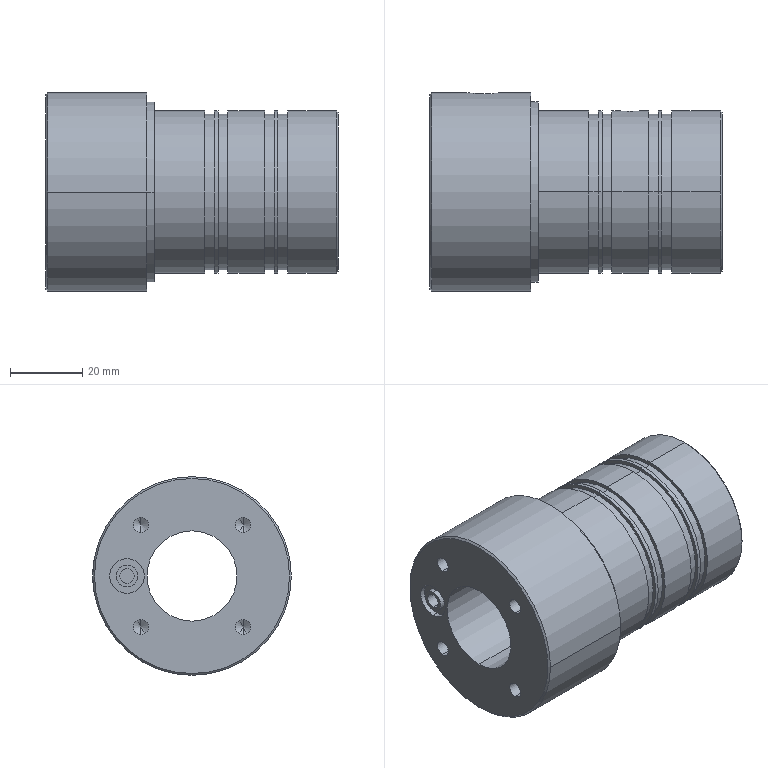Part | STEP file | 06-20 Stator core | 1 solid | 100 faces | box 81 x 55 x 55 mm | volume 107790 mm3 | cylinder 55 | cone 26 | plane 19 | commonest cylinder face diameters 45 x10 3.3 x8 4.2 x8 43 x8 6 x7 4 x4